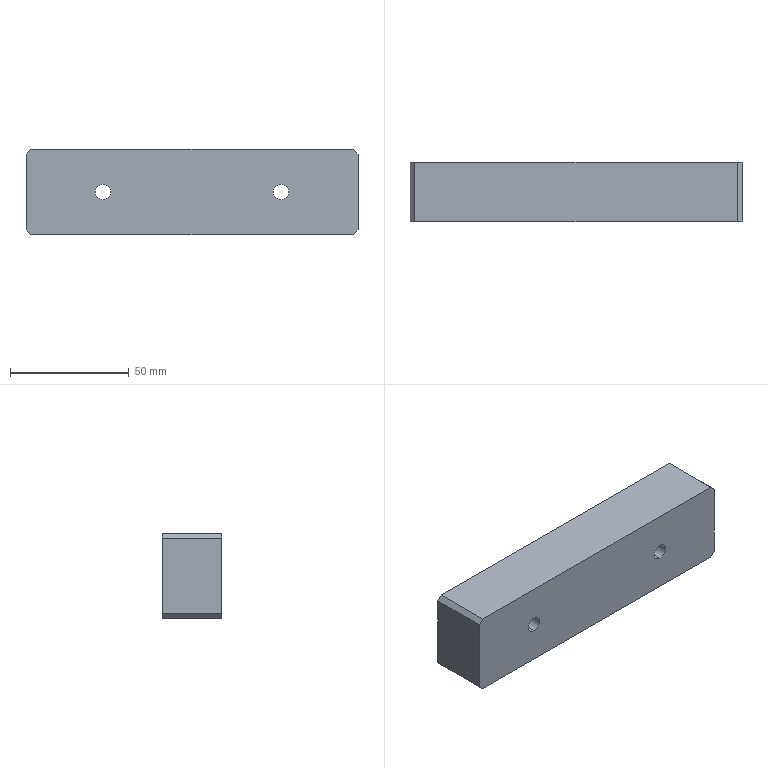Part | SolidWorks | features Chamfer 1, Extrusion 1, HoleWzd 1 | 1 solid | 20 faces | box 140 x 25 x 36 mm | volume 123238 mm3 | plane 12 | cylinder 8 | commonest cylinder face diameters 6.6 x4 11 x4
STEP:
#1=CARTESIAN_POINT('',(32.5,18.,-23.5));
#2=VERTEX_POINT('',#1);
#3=CARTESIAN_POINT('',(32.5,18.,-12.5));
#4=VERTEX_POINT('',#3);
#5=CARTESIAN_POINT('',(32.5,18.,-18.));
#6=DIRECTION('',(0.,1.,0.));
#7=DIRECTION('',(0.,0.,1.));
#8=AXIS2_PLACEMENT_3D('',#5,#6,#7);
#9=CIRCLE('',#8,5.5);
#10=EDGE_CURVE('',#2,#4,#9,.T.);
#11=ORIENTED_EDGE('',*,*,#10,.F.);
#12=CARTESIAN_POINT('',(32.5,25.,-23.5));
#13=VERTEX_POINT('',#12);
#14=CARTESIAN_POINT('',(32.5,25.,-23.5));
#15=DIRECTION('',(0.,1.,0.));
#16=VECTOR('',#15,1000.);
#17=LINE('',#14,#16);
#18=EDGE_CURVE('',#2,#13,#17,.T.);
#19=ORIENTED_EDGE('',*,*,#18,.T.);
#20=CARTESIAN_POINT('',(32.5,25.,-12.5));
#21=VERTEX_POINT('',#20);
#22=CARTESIAN_POINT('',(32.5,25.,-18.));
#23=DIRECTION('',(0.,1.,0.));
#24=DIRECTION('',(0.,0.,1.));
#25=AXIS2_PLACEMENT_3D('',#22,#23,#24);
#26=CIRCLE('',#25,5.5);
#27=EDGE_CURVE('',#13,#21,#26,.T.);
#28=ORIENTED_EDGE('',*,*,#27,.T.);
#29=CARTESIAN_POINT('',(32.5,25.,-12.5));
#30=DIRECTION('',(0.,1.,0.));
#31=VECTOR('',#30,1000.);
#32=LINE('',#29,#31);
#33=EDGE_CURVE('',#4,#21,#32,.T.);
#34=ORIENTED_EDGE('',*,*,#33,.F.);
#35=EDGE_LOOP('',(#11,#19,#28,#34));
#36=FACE_OUTER_BOUND('',#35,.T.);
#37=CARTESIAN_POINT('',(32.5,25.,-18.));
#38=DIRECTION('',(0.,1.,0.));
#39=DIRECTION('',(0.,0.,1.));
#40=AXIS2_PLACEMENT_3D('',#37,#38,#39);
#41=CYLINDRICAL_SURFACE('',#40,5.5);
#42=ADVANCED_FACE('',(#36),#41,.F.);
#43=CARTESIAN_POINT('',(32.5,0.,-21.3));
#44=VERTEX_POINT('',#43);
#45=CARTESIAN_POINT('',(32.5,0.,-14.7));
#46=VERTEX_POINT('',#45);
#47=CARTESIAN_POINT('',(32.5,0.,-18.));
#48=DIRECTION('',(0.,1.,0.));
#49=DIRECTION('',(0.,0.,1.));
#50=AXIS2_PLACEMENT_3D('',#47,#48,#49);
#51=CIRCLE('',#50,3.3);
#52=EDGE_CURVE('',#44,#46,#51,.T.);
#53=ORIENTED_EDGE('',*,*,#52,.F.);
#54=CARTESIAN_POINT('',(32.5,18.,-21.3));
#55=VERTEX_POINT('',#54);
#56=CARTESIAN_POINT('',(32.5,25.,-21.3));
#57=DIRECTION('',(0.,1.,0.));
#58=VECTOR('',#57,1000.);
#59=LINE('',#56,#58);
#60=EDGE_CURVE('',#44,#55,#59,.T.);
#61=ORIENTED_EDGE('',*,*,#60,.T.);
#62=CARTESIAN_POINT('',(32.5,18.,-14.7));
#63=VERTEX_POINT('',#62);
#64=CARTESIAN_POINT('',(32.5,18.,-18.));
#65=DIRECTION('',(0.,1.,0.));
#66=DIRECTION('',(0.,0.,1.));
#67=AXIS2_PLACEMENT_3D('',#64,#65,#66);
#68=CIRCLE('',#67,3.3);
#69=EDGE_CURVE('',#55,#63,#68,.T.);
#70=ORIENTED_EDGE('',*,*,#69,.T.);
#71=CARTESIAN_POINT('',(32.5,25.,-14.7));
#72=DIRECTION('',(0.,1.,0.));
#73=VECTOR('',#72,1000.);
#74=LINE('',#71,#73);
#75=EDGE_CURVE('',#46,#63,#74,.T.);
#76=ORIENTED_EDGE('',*,*,#75,.F.);
#77=EDGE_LOOP('',(#53,#61,#70,#76));
#78=FACE_OUTER_BOUND('',#77,.T.);
#79=CARTESIAN_POINT('',(32.5,25.,-18.));
#80=DIRECTION('',(0.,1.,0.));
#81=DIRECTION('',(0.,0.,1.));
#82=AXIS2_PLACEMENT_3D('',#79,#80,#81);
#83=CYLINDRICAL_SURFACE('',#82,3.3);
#84=ADVANCED_FACE('',(#78),#83,.F.);
#85=CARTESIAN_POINT('',(107.5,18.,-23.5));
#86=VERTEX_POINT('',#85);
#87=CARTESIAN_POINT('',(107.5,18.,-12.5));
#88=VERTEX_POINT('',#87);
#89=CARTESIAN_POINT('',(107.5,18.,-18.));
#90=DIRECTION('',(0.,1.,0.));
#91=DIRECTION('',(0.,0.,1.));
#92=AXIS2_PLACEMENT_3D('',#89,#90,#91);
#93=CIRCLE('',#92,5.5);
#94=EDGE_CURVE('',#86,#88,#93,.T.);
#95=ORIENTED_EDGE('',*,*,#94,.F.);
#96=CARTESIAN_POINT('',(107.5,25.,-23.5));
#97=VERTEX_POINT('',#96);
#98=CARTESIAN_POINT('',(107.5,25.,-23.5));
#99=DIRECTION('',(0.,1.,0.));
#100=VECTOR('',#99,1000.);
#101=LINE('',#98,#100);
#102=EDGE_CURVE('',#86,#97,#101,.T.);
#103=ORIENTED_EDGE('',*,*,#102,.T.);
#104=CARTESIAN_POINT('',(107.5,25.,-12.5));
#105=VERTEX_POINT('',#104);
#106=CARTESIAN_POINT('',(107.5,25.,-18.));
#107=DIRECTION('',(0.,1.,0.));
#108=DIRECTION('',(0.,0.,1.));
#109=AXIS2_PLACEMENT_3D('',#106,#107,#108);
#110=CIRCLE('',#109,5.5);
#111=EDGE_CURVE('',#97,#105,#110,.T.);
#112=ORIENTED_EDGE('',*,*,#111,.T.);
#113=CARTESIAN_POINT('',(107.5,25.,-12.5));
#114=DIRECTION('',(0.,1.,0.));
#115=VECTOR('',#114,1000.);
#116=LINE('',#113,#115);
#117=EDGE_CURVE('',#88,#105,#116,.T.);
#118=ORIENTED_EDGE('',*,*,#117,.F.);
#119=EDGE_LOOP('',(#95,#103,#112,#118));
#120=FACE_OUTER_BOUND('',#119,.T.);
#121=CARTESIAN_POINT('',(107.5,25.,-18.));
#122=DIRECTION('',(0.,1.,0.));
#123=DIRECTION('',(0.,0.,1.));
#124=AXIS2_PLACEMENT_3D('',#121,#122,#123);
#125=CYLINDRICAL_SURFACE('',#124,5.5);
#126=ADVANCED_FACE('',(#120),#125,.F.);
#127=CARTESIAN_POINT('',(107.5,0.,-21.3));
#128=VERTEX_POINT('',#127);
#129=CARTESIAN_POINT('',(107.5,0.,-14.7));
#130=VERTEX_POINT('',#129);
#131=CARTESIAN_POINT('',(107.5,0.,-18.));
#132=DIRECTION('',(0.,1.,0.));
#133=DIRECTION('',(0.,0.,1.));
#134=AXIS2_PLACEMENT_3D('',#131,#132,#133);
#135=CIRCLE('',#134,3.3);
#136=EDGE_CURVE('',#128,#130,#135,.T.);
#137=ORIENTED_EDGE('',*,*,#136,.F.);
#138=CARTESIAN_POINT('',(107.5,18.,-21.3));
#139=VERTEX_POINT('',#138);
#140=CARTESIAN_POINT('',(107.5,25.,-21.3));
#141=DIRECTION('',(0.,1.,0.));
#142=VECTOR('',#141,1000.);
#143=LINE('',#140,#142);
#144=EDGE_CURVE('',#128,#139,#143,.T.);
#145=ORIENTED_EDGE('',*,*,#144,.T.);
#146=CARTESIAN_POINT('',(107.5,18.,-14.7));
#147=VERTEX_POINT('',#146);
#148=CARTESIAN_POINT('',(107.5,18.,-18.));
#149=DIRECTION('',(0.,1.,0.));
#150=DIRECTION('',(0.,0.,1.));
#151=AXIS2_PLACEMENT_3D('',#148,#149,#150);
#152=CIRCLE('',#151,3.3);
#153=EDGE_CURVE('',#139,#147,#152,.T.);
#154=ORIENTED_EDGE('',*,*,#153,.T.);
#155=CARTESIAN_POINT('',(107.5,25.,-14.7));
#156=DIRECTION('',(0.,1.,0.));
#157=VECTOR('',#156,1000.);
#158=LINE('',#155,#157);
#159=EDGE_CURVE('',#130,#147,#158,.T.);
#160=ORIENTED_EDGE('',*,*,#159,.F.);
#161=EDGE_LOOP('',(#137,#145,#154,#160));
#162=FACE_OUTER_BOUND('',#161,.T.);
#163=CARTESIAN_POINT('',(107.5,25.,-18.));
#164=DIRECTION('',(0.,1.,0.));
#165=DIRECTION('',(0.,0.,1.));
#166=AXIS2_PLACEMENT_3D('',#163,#164,#165);
#167=CYLINDRICAL_SURFACE('',#166,3.3);
#168=ADVANCED_FACE('',(#162),#167,.F.);
#169=CARTESIAN_POINT('',(0.,25.,-34.));
#170=VERTEX_POINT('',#169);
#171=CARTESIAN_POINT('',(0.,25.,-2.));
#172=VERTEX_POINT('',#171);
#173=CARTESIAN_POINT('',(0.,25.,0.));
#174=DIRECTION('',(0.,0.,1.));
#175=VECTOR('',#174,1000.);
#176=LINE('',#173,#175);
#177=EDGE_CURVE('',#170,#172,#176,.T.);
#178=ORIENTED_EDGE('',*,*,#177,.F.);
#179=CARTESIAN_POINT('',(0.,0.,-34.));
#180=VERTEX_POINT('',#179);
#181=CARTESIAN_POINT('',(0.,25.,-34.));
#182=DIRECTION('',(0.,-1.,0.));
#183=VECTOR('',#182,1000.);
#184=LINE('',#181,#183);
#185=EDGE_CURVE('',#170,#180,#184,.T.);
#186=ORIENTED_EDGE('',*,*,#185,.T.);
#187=CARTESIAN_POINT('',(0.,0.,-2.));
#188=VERTEX_POINT('',#187);
#189=CARTESIAN_POINT('',(0.,0.,0.));
#190=DIRECTION('',(0.,0.,1.));
#191=VECTOR('',#190,1000.);
#192=LINE('',#189,#191);
#193=EDGE_CURVE('',#180,#188,#192,.T.);
#194=ORIENTED_EDGE('',*,*,#193,.T.);
#195=CARTESIAN_POINT('',(0.,25.,-2.));
#196=DIRECTION('',(0.,1.,0.));
#197=VECTOR('',#196,1000.);
#198=LINE('',#195,#197);
#199=EDGE_CURVE('',#188,#172,#198,.T.);
#200=ORIENTED_EDGE('',*,*,#199,.T.);
#201=EDGE_LOOP('',(#178,#186,#194,#200));
#202=FACE_OUTER_BOUND('',#201,.T.);
#203=CARTESIAN_POINT('',(0.,25.,0.));
#204=DIRECTION('',(1.,0.,0.));
#205=DIRECTION('',(0.,0.,-1.));
#206=AXIS2_PLACEMENT_3D('',#203,#204,#205);
#207=PLANE('',#206);
#208=ADVANCED_FACE('',(#202),#207,.F.);
#209=CARTESIAN_POINT('',(2.,25.,0.));
#210=VERTEX_POINT('',#209);
#211=CARTESIAN_POINT('',(138.,25.,0.));
#212=VERTEX_POINT('',#211);
#213=CARTESIAN_POINT('',(0.,25.,0.));
#214=DIRECTION('',(1.,0.,0.));
#215=VECTOR('',#214,1000.);
#216=LINE('',#213,#215);
#217=EDGE_CURVE('',#210,#212,#216,.T.);
#218=ORIENTED_EDGE('',*,*,#217,.F.);
#219=CARTESIAN_POINT('',(2.,0.,0.));
#220=VERTEX_POINT('',#219);
#221=CARTESIAN_POINT('',(2.,25.,0.));
#222=DIRECTION('',(0.,-1.,0.));
#223=VECTOR('',#222,1000.);
#224=LINE('',#221,#223);
#225=EDGE_CURVE('',#210,#220,#224,.T.);
#226=ORIENTED_EDGE('',*,*,#225,.T.);
#227=CARTESIAN_POINT('',(138.,0.,0.));
#228=VERTEX_POINT('',#227);
#229=CARTESIAN_POINT('',(0.,0.,0.));
#230=DIRECTION('',(1.,0.,0.));
#231=VECTOR('',#230,1000.);
#232=LINE('',#229,#231);
#233=EDGE_CURVE('',#220,#228,#232,.T.);
#234=ORIENTED_EDGE('',*,*,#233,.T.);
#235=CARTESIAN_POINT('',(138.,25.,0.));
#236=DIRECTION('',(0.,1.,0.));
#237=VECTOR('',#236,1000.);
#238=LINE('',#235,#237);
#239=EDGE_CURVE('',#228,#212,#238,.T.);
#240=ORIENTED_EDGE('',*,*,#239,.T.);
#241=EDGE_LOOP('',(#218,#226,#234,#240));
#242=FACE_OUTER_BOUND('',#241,.T.);
#243=CARTESIAN_POINT('',(0.,25.,0.));
#244=DIRECTION('',(0.,0.,-1.));
#245=DIRECTION('',(-1.,0.,0.));
#246=AXIS2_PLACEMENT_3D('',#243,#244,#245);
#247=PLANE('',#246);
#248=ADVANCED_FACE('',(#242),#247,.F.);
#249=CARTESIAN_POINT('',(140.,0.,-2.));
#250=VERTEX_POINT('',#249);
#251=CARTESIAN_POINT('',(140.,0.,-34.));
#252=VERTEX_POINT('',#251);
#253=CARTESIAN_POINT('',(140.,0.,0.));
#254=DIRECTION('',(0.,0.,-1.));
#255=VECTOR('',#254,1000.);
#256=LINE('',#253,#255);
#257=EDGE_CURVE('',#250,#252,#256,.T.);
#258=ORIENTED_EDGE('',*,*,#257,.T.);
#259=CARTESIAN_POINT('',(140.,25.,-34.));
#260=VERTEX_POINT('',#259);
#261=CARTESIAN_POINT('',(140.,25.,-34.));
#262=DIRECTION('',(0.,1.,0.));
#263=VECTOR('',#262,1000.);
#264=LINE('',#261,#263);
#265=EDGE_CURVE('',#252,#260,#264,.T.);
#266=ORIENTED_EDGE('',*,*,#265,.T.);
#267=CARTESIAN_POINT('',(140.,25.,-2.));
#268=VERTEX_POINT('',#267);
#269=CARTESIAN_POINT('',(140.,25.,0.));
#270=DIRECTION('',(0.,0.,-1.));
#271=VECTOR('',#270,1000.);
#272=LINE('',#269,#271);
#273=EDGE_CURVE('',#268,#260,#272,.T.);
#274=ORIENTED_EDGE('',*,*,#273,.F.);
#275=CARTESIAN_POINT('',(140.,25.,-2.));
#276=DIRECTION('',(0.,-1.,0.));
#277=VECTOR('',#276,1000.);
#278=LINE('',#275,#277);
#279=EDGE_CURVE('',#268,#250,#278,.T.);
#280=ORIENTED_EDGE('',*,*,#279,.T.);
#281=EDGE_LOOP('',(#258,#266,#274,#280));
#282=FACE_OUTER_BOUND('',#281,.T.);
#283=CARTESIAN_POINT('',(140.,25.,0.));
#284=DIRECTION('',(-1.,0.,0.));
#285=DIRECTION('',(0.,0.,1.));
#286=AXIS2_PLACEMENT_3D('',#283,#284,#285);
#287=PLANE('',#286);
#288=ADVANCED_FACE('',(#282),#287,.F.);
#289=CARTESIAN_POINT('',(138.,0.,-36.));
#290=VERTEX_POINT('',#289);
#291=CARTESIAN_POINT('',(2.,0.,-36.));
#292=VERTEX_POINT('',#291);
#293=CARTESIAN_POINT('',(0.,0.,-36.));
#294=DIRECTION('',(-1.,0.,0.));
#295=VECTOR('',#294,1000.);
#296=LINE('',#293,#295);
#297=EDGE_CURVE('',#290,#292,#296,.T.);
#298=ORIENTED_EDGE('',*,*,#297,.T.);
#299=CARTESIAN_POINT('',(2.,25.,-36.));
#300=VERTEX_POINT('',#299);
#301=CARTESIAN_POINT('',(2.,25.,-36.));
#302=DIRECTION('',(0.,1.,0.));
#303=VECTOR('',#302,1000.);
#304=LINE('',#301,#303);
#305=EDGE_CURVE('',#292,#300,#304,.T.);
#306=ORIENTED_EDGE('',*,*,#305,.T.);
#307=CARTESIAN_POINT('',(138.,25.,-36.));
#308=VERTEX_POINT('',#307);
#309=CARTESIAN_POINT('',(0.,25.,-36.));
#310=DIRECTION('',(-1.,0.,0.));
#311=VECTOR('',#310,1000.);
#312=LINE('',#309,#311);
#313=EDGE_CURVE('',#308,#300,#312,.T.);
#314=ORIENTED_EDGE('',*,*,#313,.F.);
#315=CARTESIAN_POINT('',(138.,25.,-36.));
#316=DIRECTION('',(0.,-1.,0.));
#317=VECTOR('',#316,1000.);
#318=LINE('',#315,#317);
#319=EDGE_CURVE('',#308,#290,#318,.T.);
#320=ORIENTED_EDGE('',*,*,#319,.T.);
#321=EDGE_LOOP('',(#298,#306,#314,#320));
#322=FACE_OUTER_BOUND('',#321,.T.);
#323=CARTESIAN_POINT('',(0.,25.,-36.));
#324=DIRECTION('',(0.,0.,1.));
#325=DIRECTION('',(1.,0.,0.));
#326=AXIS2_PLACEMENT_3D('',#323,#324,#325);
#327=PLANE('',#326);
#328=ADVANCED_FACE('',(#322),#327,.F.);
#329=CARTESIAN_POINT('',(32.5,25.,-18.));
#330=DIRECTION('',(0.,1.,0.));
#331=DIRECTION('',(0.,0.,1.));
#332=AXIS2_PLACEMENT_3D('',#329,#330,#331);
#333=CIRCLE('',#332,5.5);
#334=EDGE_CURVE('',#21,#13,#333,.T.);
#335=ORIENTED_EDGE('',*,*,#334,.F.);
#336=ORIENTED_EDGE('',*,*,#27,.F.);
#337=EDGE_LOOP('',(#335,#336));
#338=FACE_BOUND('',#337,.T.);
#339=CARTESIAN_POINT('',(107.5,25.,-18.));
#340=DIRECTION('',(0.,1.,0.));
#341=DIRECTION('',(0.,0.,1.));
#342=AXIS2_PLACEMENT_3D('',#339,#340,#341);
#343=CIRCLE('',#342,5.5);
#344=EDGE_CURVE('',#105,#97,#343,.T.);
#345=ORIENTED_EDGE('',*,*,#344,.F.);
#346=ORIENTED_EDGE('',*,*,#111,.F.);
#347=EDGE_LOOP('',(#345,#346));
#348=FACE_BOUND('',#347,.T.);
#349=ORIENTED_EDGE('',*,*,#313,.T.);
#350=CARTESIAN_POINT('',(0.,25.,-34.));
#351=DIRECTION('',(-0.7071,0.,0.7071));
#352=VECTOR('',#351,1000.);
#353=LINE('',#350,#352);
#354=EDGE_CURVE('',#300,#170,#353,.T.);
#355=ORIENTED_EDGE('',*,*,#354,.T.);
#356=ORIENTED_EDGE('',*,*,#177,.T.);
#357=CARTESIAN_POINT('',(2.,25.,0.));
#358=DIRECTION('',(0.7071,0.,0.7071));
#359=VECTOR('',#358,1000.);
#360=LINE('',#357,#359);
#361=EDGE_CURVE('',#172,#210,#360,.T.);
#362=ORIENTED_EDGE('',*,*,#361,.T.);
#363=ORIENTED_EDGE('',*,*,#217,.T.);
#364=CARTESIAN_POINT('',(140.,25.,-2.));
#365=DIRECTION('',(0.7071,0.,-0.7071));
#366=VECTOR('',#365,1000.);
#367=LINE('',#364,#366);
#368=EDGE_CURVE('',#212,#268,#367,.T.);
#369=ORIENTED_EDGE('',*,*,#368,.T.);
#370=ORIENTED_EDGE('',*,*,#273,.T.);
#371=CARTESIAN_POINT('',(138.,25.,-36.));
#372=DIRECTION('',(-0.7071,0.,-0.7071));
#373=VECTOR('',#372,1000.);
#374=LINE('',#371,#373);
#375=EDGE_CURVE('',#260,#308,#374,.T.);
#376=ORIENTED_EDGE('',*,*,#375,.T.);
#377=EDGE_LOOP('',(#349,#355,#356,#362,#363,#369,#370,#376));
#378=FACE_OUTER_BOUND('',#377,.T.);
#379=CARTESIAN_POINT('',(0.,25.,0.));
#380=DIRECTION('',(0.,-1.,0.));
#381=DIRECTION('',(0.,0.,-1.));
#382=AXIS2_PLACEMENT_3D('',#379,#380,#381);
#383=PLANE('',#382);
#384=ADVANCED_FACE('',(#338,#348,#378),#383,.F.);
#385=CARTESIAN_POINT('',(32.5,0.,-18.));
#386=DIRECTION('',(0.,1.,0.));
#387=DIRECTION('',(0.,0.,1.));
#388=AXIS2_PLACEMENT_3D('',#385,#386,#387);
#389=CIRCLE('',#388,3.3);
#390=EDGE_CURVE('',#46,#44,#389,.T.);
#391=ORIENTED_EDGE('',*,*,#390,.T.);
#392=ORIENTED_EDGE('',*,*,#52,.T.);
#393=EDGE_LOOP('',(#391,#392));
#394=FACE_BOUND('',#393,.T.);
#395=CARTESIAN_POINT('',(107.5,0.,-18.));
#396=DIRECTION('',(0.,1.,0.));
#397=DIRECTION('',(0.,0.,1.));
#398=AXIS2_PLACEMENT_3D('',#395,#396,#397);
#399=CIRCLE('',#398,3.3);
#400=EDGE_CURVE('',#130,#128,#399,.T.);
#401=ORIENTED_EDGE('',*,*,#400,.T.);
#402=ORIENTED_EDGE('',*,*,#136,.T.);
#403=EDGE_LOOP('',(#401,#402));
#404=FACE_BOUND('',#403,.T.);
#405=ORIENTED_EDGE('',*,*,#193,.F.);
#406=CARTESIAN_POINT('',(-17.,0.,-17.));
#407=DIRECTION('',(0.7071,0.,-0.7071));
#408=VECTOR('',#407,1000.);
#409=LINE('',#406,#408);
#410=EDGE_CURVE('',#180,#292,#409,.T.);
#411=ORIENTED_EDGE('',*,*,#410,.T.);
#412=ORIENTED_EDGE('',*,*,#297,.F.);
#413=CARTESIAN_POINT('',(87.,0.,-87.));
#414=DIRECTION('',(0.7071,0.,0.7071));
#415=VECTOR('',#414,1000.);
#416=LINE('',#413,#415);
#417=EDGE_CURVE('',#290,#252,#416,.T.);
#418=ORIENTED_EDGE('',*,*,#417,.T.);
#419=ORIENTED_EDGE('',*,*,#257,.F.);
#420=CARTESIAN_POINT('',(69.,0.,69.));
#421=DIRECTION('',(-0.7071,0.,0.7071));
#422=VECTOR('',#421,1000.);
#423=LINE('',#420,#422);
#424=EDGE_CURVE('',#250,#228,#423,.T.);
#425=ORIENTED_EDGE('',*,*,#424,.T.);
#426=ORIENTED_EDGE('',*,*,#233,.F.);
#427=CARTESIAN_POINT('',(1.,0.,-1.));
#428=DIRECTION('',(-0.7071,0.,-0.7071));
#429=VECTOR('',#428,1000.);
#430=LINE('',#427,#429);
#431=EDGE_CURVE('',#220,#188,#430,.T.);
#432=ORIENTED_EDGE('',*,*,#431,.T.);
#433=EDGE_LOOP('',(#405,#411,#412,#418,#419,#425,#426,#432));
#434=FACE_OUTER_BOUND('',#433,.T.);
#435=CARTESIAN_POINT('',(0.,0.,0.));
#436=DIRECTION('',(0.,-1.,0.));
#437=DIRECTION('',(0.,0.,-1.));
#438=AXIS2_PLACEMENT_3D('',#435,#436,#437);
#439=PLANE('',#438);
#440=ADVANCED_FACE('',(#394,#404,#434),#439,.T.);
#441=ORIENTED_EDGE('',*,*,#144,.F.);
#442=ORIENTED_EDGE('',*,*,#400,.F.);
#443=ORIENTED_EDGE('',*,*,#159,.T.);
#444=CARTESIAN_POINT('',(107.5,18.,-18.));
#445=DIRECTION('',(0.,1.,0.));
#446=DIRECTION('',(0.,0.,1.));
#447=AXIS2_PLACEMENT_3D('',#444,#445,#446);
#448=CIRCLE('',#447,3.3);
#449=EDGE_CURVE('',#147,#139,#448,.T.);
#450=ORIENTED_EDGE('',*,*,#449,.T.);
#451=EDGE_LOOP('',(#441,#442,#443,#450));
#452=FACE_OUTER_BOUND('',#451,.T.);
#453=CARTESIAN_POINT('',(107.5,25.,-18.));
#454=DIRECTION('',(0.,1.,0.));
#455=DIRECTION('',(0.,0.,1.));
#456=AXIS2_PLACEMENT_3D('',#453,#454,#455);
#457=CYLINDRICAL_SURFACE('',#456,3.3);
#458=ADVANCED_FACE('',(#452),#457,.F.);
#459=ORIENTED_EDGE('',*,*,#449,.F.);
#460=ORIENTED_EDGE('',*,*,#153,.F.);
#461=EDGE_LOOP('',(#459,#460));
#462=FACE_BOUND('',#461,.T.);
#463=CARTESIAN_POINT('',(107.5,18.,-18.));
#464=DIRECTION('',(0.,1.,0.));
#465=DIRECTION('',(0.,0.,1.));
#466=AXIS2_PLACEMENT_3D('',#463,#464,#465);
#467=CIRCLE('',#466,5.5);
#468=EDGE_CURVE('',#88,#86,#467,.T.);
#469=ORIENTED_EDGE('',*,*,#468,.T.);
#470=ORIENTED_EDGE('',*,*,#94,.T.);
#471=EDGE_LOOP('',(#469,#470));
#472=FACE_OUTER_BOUND('',#471,.T.);
#473=CARTESIAN_POINT('',(110.8,18.,-18.));
#474=DIRECTION('',(0.,-1.,0.));
#475=DIRECTION('',(0.,0.,-1.));
#476=AXIS2_PLACEMENT_3D('',#473,#474,#475);
#477=PLANE('',#476);
#478=ADVANCED_FACE('',(#462,#472),#477,.F.);
#479=ORIENTED_EDGE('',*,*,#102,.F.);
#480=ORIENTED_EDGE('',*,*,#468,.F.);
#481=ORIENTED_EDGE('',*,*,#117,.T.);
#482=ORIENTED_EDGE('',*,*,#344,.T.);
#483=EDGE_LOOP('',(#479,#480,#481,#482));
#484=FACE_OUTER_BOUND('',#483,.T.);
#485=CARTESIAN_POINT('',(107.5,25.,-18.));
#486=DIRECTION('',(0.,1.,0.));
#487=DIRECTION('',(0.,0.,1.));
#488=AXIS2_PLACEMENT_3D('',#485,#486,#487);
#489=CYLINDRICAL_SURFACE('',#488,5.5);
#490=ADVANCED_FACE('',(#484),#489,.F.);
#491=ORIENTED_EDGE('',*,*,#60,.F.);
#492=ORIENTED_EDGE('',*,*,#390,.F.);
#493=ORIENTED_EDGE('',*,*,#75,.T.);
#494=CARTESIAN_POINT('',(32.5,18.,-18.));
#495=DIRECTION('',(0.,1.,0.));
#496=DIRECTION('',(0.,0.,1.));
#497=AXIS2_PLACEMENT_3D('',#494,#495,#496);
#498=CIRCLE('',#497,3.3);
#499=EDGE_CURVE('',#63,#55,#498,.T.);
#500=ORIENTED_EDGE('',*,*,#499,.T.);
#501=EDGE_LOOP('',(#491,#492,#493,#500));
#502=FACE_OUTER_BOUND('',#501,.T.);
#503=CARTESIAN_POINT('',(32.5,25.,-18.));
#504=DIRECTION('',(0.,1.,0.));
#505=DIRECTION('',(0.,0.,1.));
#506=AXIS2_PLACEMENT_3D('',#503,#504,#505);
#507=CYLINDRICAL_SURFACE('',#506,3.3);
#508=ADVANCED_FACE('',(#502),#507,.F.);
#509=ORIENTED_EDGE('',*,*,#499,.F.);
#510=ORIENTED_EDGE('',*,*,#69,.F.);
#511=EDGE_LOOP('',(#509,#510));
#512=FACE_BOUND('',#511,.T.);
#513=CARTESIAN_POINT('',(32.5,18.,-18.));
#514=DIRECTION('',(0.,1.,0.));
#515=DIRECTION('',(0.,0.,1.));
#516=AXIS2_PLACEMENT_3D('',#513,#514,#515);
#517=CIRCLE('',#516,5.5);
#518=EDGE_CURVE('',#4,#2,#517,.T.);
#519=ORIENTED_EDGE('',*,*,#518,.T.);
#520=ORIENTED_EDGE('',*,*,#10,.T.);
#521=EDGE_LOOP('',(#519,#520));
#522=FACE_OUTER_BOUND('',#521,.T.);
#523=CARTESIAN_POINT('',(35.8,18.,-18.));
#524=DIRECTION('',(0.,-1.,0.));
#525=DIRECTION('',(0.,0.,-1.));
#526=AXIS2_PLACEMENT_3D('',#523,#524,#525);
#527=PLANE('',#526);
#528=ADVANCED_FACE('',(#512,#522),#527,.F.);
#529=ORIENTED_EDGE('',*,*,#18,.F.);
#530=ORIENTED_EDGE('',*,*,#518,.F.);
#531=ORIENTED_EDGE('',*,*,#33,.T.);
#532=ORIENTED_EDGE('',*,*,#334,.T.);
#533=EDGE_LOOP('',(#529,#530,#531,#532));
#534=FACE_OUTER_BOUND('',#533,.T.);
#535=CARTESIAN_POINT('',(32.5,25.,-18.));
#536=DIRECTION('',(0.,1.,0.));
#537=DIRECTION('',(0.,0.,1.));
#538=AXIS2_PLACEMENT_3D('',#535,#536,#537);
#539=CYLINDRICAL_SURFACE('',#538,5.5);
#540=ADVANCED_FACE('',(#534),#539,.F.);
#541=ORIENTED_EDGE('',*,*,#354,.F.);
#542=ORIENTED_EDGE('',*,*,#305,.F.);
#543=ORIENTED_EDGE('',*,*,#410,.F.);
#544=ORIENTED_EDGE('',*,*,#185,.F.);
#545=EDGE_LOOP('',(#541,#542,#543,#544));
#546=FACE_OUTER_BOUND('',#545,.T.);
#547=CARTESIAN_POINT('',(0.,25.,-34.));
#548=DIRECTION('',(0.7071,0.,0.7071));
#549=DIRECTION('',(0.,-1.,0.));
#550=AXIS2_PLACEMENT_3D('',#547,#548,#549);
#551=PLANE('',#550);
#552=ADVANCED_FACE('',(#546),#551,.F.);
#553=ORIENTED_EDGE('',*,*,#361,.F.);
#554=ORIENTED_EDGE('',*,*,#199,.F.);
#555=ORIENTED_EDGE('',*,*,#431,.F.);
#556=ORIENTED_EDGE('',*,*,#225,.F.);
#557=EDGE_LOOP('',(#553,#554,#555,#556));
#558=FACE_OUTER_BOUND('',#557,.T.);
#559=CARTESIAN_POINT('',(2.,25.,0.));
#560=DIRECTION('',(0.7071,0.,-0.7071));
#561=DIRECTION('',(0.,-1.,0.));
#562=AXIS2_PLACEMENT_3D('',#559,#560,#561);
#563=PLANE('',#562);
#564=ADVANCED_FACE('',(#558),#563,.F.);
#565=ORIENTED_EDGE('',*,*,#375,.F.);
#566=ORIENTED_EDGE('',*,*,#265,.F.);
#567=ORIENTED_EDGE('',*,*,#417,.F.);
#568=ORIENTED_EDGE('',*,*,#319,.F.);
#569=EDGE_LOOP('',(#565,#566,#567,#568));
#570=FACE_OUTER_BOUND('',#569,.T.);
#571=CARTESIAN_POINT('',(138.,25.,-36.));
#572=DIRECTION('',(-0.7071,0.,0.7071));
#573=DIRECTION('',(0.,-1.,0.));
#574=AXIS2_PLACEMENT_3D('',#571,#572,#573);
#575=PLANE('',#574);
#576=ADVANCED_FACE('',(#570),#575,.F.);
#577=ORIENTED_EDGE('',*,*,#368,.F.);
#578=ORIENTED_EDGE('',*,*,#239,.F.);
#579=ORIENTED_EDGE('',*,*,#424,.F.);
#580=ORIENTED_EDGE('',*,*,#279,.F.);
#581=EDGE_LOOP('',(#577,#578,#579,#580));
#582=FACE_OUTER_BOUND('',#581,.T.);
#583=CARTESIAN_POINT('',(140.,25.,-2.));
#584=DIRECTION('',(-0.7071,0.,-0.7071));
#585=DIRECTION('',(0.,-1.,0.));
#586=AXIS2_PLACEMENT_3D('',#583,#584,#585);
#587=PLANE('',#586);
#588=ADVANCED_FACE('',(#582),#587,.F.);
#589=CLOSED_SHELL('',(#42,#84,#126,#168,#208,#248,#288,#328,#384,#440,#458,#478,#490,#508,#528,#540,#552,#564,#576,#588));
#590=MANIFOLD_SOLID_BREP('',#589);
#591=CARTESIAN_POINT('',(0.,0.,0.));
#592=DIRECTION('',(0.,0.,1.));
#593=DIRECTION('',(1.,0.,0.));
#594=AXIS2_PLACEMENT_3D('',#591,#592,#593);
#595=(LENGTH_UNIT()NAMED_UNIT(*)SI_UNIT(.MILLI.,.METRE.));
#596=UNCERTAINTY_MEASURE_WITH_UNIT(LENGTH_MEASURE(0.00001),#595,'','');
#597=(NAMED_UNIT(*)PLANE_ANGLE_UNIT()SI_UNIT($,.RADIAN.));
#598=(NAMED_UNIT(*)SI_UNIT($,.STERADIAN.)SOLID_ANGLE_UNIT());
#599=(GEOMETRIC_REPRESENTATION_CONTEXT(3)GLOBAL_UNCERTAINTY_ASSIGNED_CONTEXT((#596))GLOBAL_UNIT_ASSIGNED_CONTEXT((#595,#597,#598))REPRESENTATION_CONTEXT('',''));
#600=ADVANCED_BREP_SHAPE_REPRESENTATION('',(#590,#594),#599);